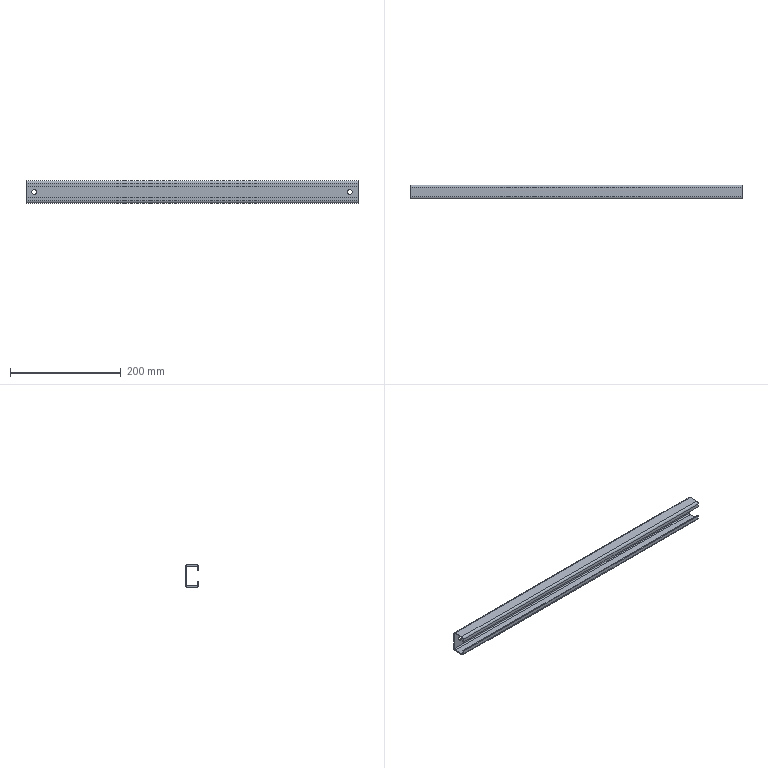Part | SolidWorks | features BaseBody 1 | 1 solid | 26 faces | box 600 x 25 x 40 mm | volume 115965 mm3 | plane 14 | cylinder 12 | commonest cylinder face diameters 4 x4 8 x4 9 x4
STEP:
#1=CARTESIAN_POINT('',(-285.,2.,4.5));
#2=VERTEX_POINT('',#1);
#3=CARTESIAN_POINT('',(-285.,2.,-4.5));
#4=VERTEX_POINT('',#3);
#5=CARTESIAN_POINT('',(-285.,2.,0.));
#6=DIRECTION('',(0.,-1.,0.));
#7=DIRECTION('',(0.,0.,-1.));
#8=AXIS2_PLACEMENT_3D('',#5,#6,#7);
#9=CIRCLE('',#8,4.5);
#10=EDGE_CURVE('',#2,#4,#9,.T.);
#11=ORIENTED_EDGE('',*,*,#10,.F.);
#12=CARTESIAN_POINT('',(-285.,0.,4.5));
#13=VERTEX_POINT('',#12);
#14=CARTESIAN_POINT('',(-285.,2.,4.5));
#15=DIRECTION('',(0.,-1.,0.));
#16=VECTOR('',#15,1000.);
#17=LINE('',#14,#16);
#18=EDGE_CURVE('',#2,#13,#17,.T.);
#19=ORIENTED_EDGE('',*,*,#18,.T.);
#20=CARTESIAN_POINT('',(-285.,0.,-4.5));
#21=VERTEX_POINT('',#20);
#22=CARTESIAN_POINT('',(-285.,0.,0.));
#23=DIRECTION('',(0.,-1.,0.));
#24=DIRECTION('',(0.,0.,-1.));
#25=AXIS2_PLACEMENT_3D('',#22,#23,#24);
#26=CIRCLE('',#25,4.5);
#27=EDGE_CURVE('',#13,#21,#26,.T.);
#28=ORIENTED_EDGE('',*,*,#27,.T.);
#29=CARTESIAN_POINT('',(-285.,2.,-4.5));
#30=DIRECTION('',(0.,-1.,0.));
#31=VECTOR('',#30,1000.);
#32=LINE('',#29,#31);
#33=EDGE_CURVE('',#4,#21,#32,.T.);
#34=ORIENTED_EDGE('',*,*,#33,.F.);
#35=EDGE_LOOP('',(#11,#19,#28,#34));
#36=FACE_OUTER_BOUND('',#35,.T.);
#37=CARTESIAN_POINT('',(-285.,2.,0.));
#38=DIRECTION('',(0.,-1.,0.));
#39=DIRECTION('',(0.,0.,-1.));
#40=AXIS2_PLACEMENT_3D('',#37,#38,#39);
#41=CYLINDRICAL_SURFACE('',#40,4.5);
#42=ADVANCED_FACE('',(#36),#41,.F.);
#43=CARTESIAN_POINT('',(285.,2.,4.5));
#44=VERTEX_POINT('',#43);
#45=CARTESIAN_POINT('',(285.,2.,-4.5));
#46=VERTEX_POINT('',#45);
#47=CARTESIAN_POINT('',(285.,2.,0.));
#48=DIRECTION('',(0.,-1.,0.));
#49=DIRECTION('',(0.,0.,-1.));
#50=AXIS2_PLACEMENT_3D('',#47,#48,#49);
#51=CIRCLE('',#50,4.5);
#52=EDGE_CURVE('',#44,#46,#51,.T.);
#53=ORIENTED_EDGE('',*,*,#52,.F.);
#54=CARTESIAN_POINT('',(285.,0.,4.5));
#55=VERTEX_POINT('',#54);
#56=CARTESIAN_POINT('',(285.,2.,4.5));
#57=DIRECTION('',(0.,-1.,0.));
#58=VECTOR('',#57,1000.);
#59=LINE('',#56,#58);
#60=EDGE_CURVE('',#44,#55,#59,.T.);
#61=ORIENTED_EDGE('',*,*,#60,.T.);
#62=CARTESIAN_POINT('',(285.,0.,-4.5));
#63=VERTEX_POINT('',#62);
#64=CARTESIAN_POINT('',(285.,0.,0.));
#65=DIRECTION('',(0.,-1.,0.));
#66=DIRECTION('',(0.,0.,-1.));
#67=AXIS2_PLACEMENT_3D('',#64,#65,#66);
#68=CIRCLE('',#67,4.5);
#69=EDGE_CURVE('',#55,#63,#68,.T.);
#70=ORIENTED_EDGE('',*,*,#69,.T.);
#71=CARTESIAN_POINT('',(285.,2.,-4.5));
#72=DIRECTION('',(0.,-1.,0.));
#73=VECTOR('',#72,1000.);
#74=LINE('',#71,#73);
#75=EDGE_CURVE('',#46,#63,#74,.T.);
#76=ORIENTED_EDGE('',*,*,#75,.F.);
#77=EDGE_LOOP('',(#53,#61,#70,#76));
#78=FACE_OUTER_BOUND('',#77,.T.);
#79=CARTESIAN_POINT('',(285.,2.,0.));
#80=DIRECTION('',(0.,-1.,0.));
#81=DIRECTION('',(0.,0.,-1.));
#82=AXIS2_PLACEMENT_3D('',#79,#80,#81);
#83=CYLINDRICAL_SURFACE('',#82,4.5);
#84=ADVANCED_FACE('',(#78),#83,.F.);
#85=CARTESIAN_POINT('',(-285.,0.,0.));
#86=DIRECTION('',(0.,-1.,0.));
#87=DIRECTION('',(0.,0.,-1.));
#88=AXIS2_PLACEMENT_3D('',#85,#86,#87);
#89=CIRCLE('',#88,4.5);
#90=EDGE_CURVE('',#21,#13,#89,.T.);
#91=ORIENTED_EDGE('',*,*,#90,.F.);
#92=ORIENTED_EDGE('',*,*,#27,.F.);
#93=EDGE_LOOP('',(#91,#92));
#94=FACE_BOUND('',#93,.T.);
#95=CARTESIAN_POINT('',(285.,0.,0.));
#96=DIRECTION('',(0.,-1.,0.));
#97=DIRECTION('',(0.,0.,-1.));
#98=AXIS2_PLACEMENT_3D('',#95,#96,#97);
#99=CIRCLE('',#98,4.5);
#100=EDGE_CURVE('',#63,#55,#99,.T.);
#101=ORIENTED_EDGE('',*,*,#100,.F.);
#102=ORIENTED_EDGE('',*,*,#69,.F.);
#103=EDGE_LOOP('',(#101,#102));
#104=FACE_BOUND('',#103,.T.);
#105=CARTESIAN_POINT('',(300.,0.,16.));
#106=VERTEX_POINT('',#105);
#107=CARTESIAN_POINT('',(300.,0.,-16.));
#108=VERTEX_POINT('',#107);
#109=CARTESIAN_POINT('',(300.,0.,0.));
#110=DIRECTION('',(0.,0.,-1.));
#111=VECTOR('',#110,1000.);
#112=LINE('',#109,#111);
#113=EDGE_CURVE('',#106,#108,#112,.T.);
#114=ORIENTED_EDGE('',*,*,#113,.F.);
#115=CARTESIAN_POINT('',(-300.,0.,16.));
#116=VERTEX_POINT('',#115);
#117=CARTESIAN_POINT('',(0.,0.,16.));
#118=DIRECTION('',(1.,0.,0.));
#119=VECTOR('',#118,1000.);
#120=LINE('',#117,#119);
#121=EDGE_CURVE('',#116,#106,#120,.T.);
#122=ORIENTED_EDGE('',*,*,#121,.F.);
#123=CARTESIAN_POINT('',(-300.,0.,-16.));
#124=VERTEX_POINT('',#123);
#125=CARTESIAN_POINT('',(-300.,0.,0.));
#126=DIRECTION('',(0.,0.,1.));
#127=VECTOR('',#126,1000.);
#128=LINE('',#125,#127);
#129=EDGE_CURVE('',#124,#116,#128,.T.);
#130=ORIENTED_EDGE('',*,*,#129,.F.);
#131=CARTESIAN_POINT('',(0.,0.,-16.));
#132=DIRECTION('',(-1.,0.,0.));
#133=VECTOR('',#132,1000.);
#134=LINE('',#131,#133);
#135=EDGE_CURVE('',#108,#124,#134,.T.);
#136=ORIENTED_EDGE('',*,*,#135,.F.);
#137=EDGE_LOOP('',(#114,#122,#130,#136));
#138=FACE_OUTER_BOUND('',#137,.T.);
#139=CARTESIAN_POINT('',(0.,0.,0.));
#140=DIRECTION('',(0.,1.,0.));
#141=DIRECTION('',(0.,0.,1.));
#142=AXIS2_PLACEMENT_3D('',#139,#140,#141);
#143=PLANE('',#142);
#144=ADVANCED_FACE('',(#94,#104,#138),#143,.F.);
#145=ORIENTED_EDGE('',*,*,#18,.F.);
#146=CARTESIAN_POINT('',(-285.,2.,0.));
#147=DIRECTION('',(0.,-1.,0.));
#148=DIRECTION('',(0.,0.,-1.));
#149=AXIS2_PLACEMENT_3D('',#146,#147,#148);
#150=CIRCLE('',#149,4.5);
#151=EDGE_CURVE('',#4,#2,#150,.T.);
#152=ORIENTED_EDGE('',*,*,#151,.F.);
#153=ORIENTED_EDGE('',*,*,#33,.T.);
#154=ORIENTED_EDGE('',*,*,#90,.T.);
#155=EDGE_LOOP('',(#145,#152,#153,#154));
#156=FACE_OUTER_BOUND('',#155,.T.);
#157=CARTESIAN_POINT('',(-285.,2.,0.));
#158=DIRECTION('',(0.,-1.,0.));
#159=DIRECTION('',(0.,0.,-1.));
#160=AXIS2_PLACEMENT_3D('',#157,#158,#159);
#161=CYLINDRICAL_SURFACE('',#160,4.5);
#162=ADVANCED_FACE('',(#156),#161,.F.);
#163=ORIENTED_EDGE('',*,*,#60,.F.);
#164=CARTESIAN_POINT('',(285.,2.,0.));
#165=DIRECTION('',(0.,-1.,0.));
#166=DIRECTION('',(0.,0.,-1.));
#167=AXIS2_PLACEMENT_3D('',#164,#165,#166);
#168=CIRCLE('',#167,4.5);
#169=EDGE_CURVE('',#46,#44,#168,.T.);
#170=ORIENTED_EDGE('',*,*,#169,.F.);
#171=ORIENTED_EDGE('',*,*,#75,.T.);
#172=ORIENTED_EDGE('',*,*,#100,.T.);
#173=EDGE_LOOP('',(#163,#170,#171,#172));
#174=FACE_OUTER_BOUND('',#173,.T.);
#175=CARTESIAN_POINT('',(285.,2.,0.));
#176=DIRECTION('',(0.,-1.,0.));
#177=DIRECTION('',(0.,0.,-1.));
#178=AXIS2_PLACEMENT_3D('',#175,#176,#177);
#179=CYLINDRICAL_SURFACE('',#178,4.5);
#180=ADVANCED_FACE('',(#174),#179,.F.);
#181=ORIENTED_EDGE('',*,*,#135,.T.);
#182=CARTESIAN_POINT('',(-300.,-2.,-18.));
#183=VERTEX_POINT('',#182);
#184=CARTESIAN_POINT('',(-300.,-2.,-16.));
#185=DIRECTION('',(1.,0.,0.));
#186=DIRECTION('',(0.,0.,-1.));
#187=AXIS2_PLACEMENT_3D('',#184,#185,#186);
#188=CIRCLE('',#187,2.);
#189=EDGE_CURVE('',#183,#124,#188,.T.);
#190=ORIENTED_EDGE('',*,*,#189,.F.);
#191=CARTESIAN_POINT('',(300.,-2.,-18.));
#192=VERTEX_POINT('',#191);
#193=CARTESIAN_POINT('',(-300.,-2.,-18.));
#194=DIRECTION('',(-1.,0.,0.));
#195=VECTOR('',#194,1000.);
#196=LINE('',#193,#195);
#197=EDGE_CURVE('',#192,#183,#196,.T.);
#198=ORIENTED_EDGE('',*,*,#197,.F.);
#199=CARTESIAN_POINT('',(300.,-2.,-16.));
#200=DIRECTION('',(-1.,0.,0.));
#201=DIRECTION('',(0.,0.,-1.));
#202=AXIS2_PLACEMENT_3D('',#199,#200,#201);
#203=CIRCLE('',#202,2.);
#204=EDGE_CURVE('',#108,#192,#203,.T.);
#205=ORIENTED_EDGE('',*,*,#204,.F.);
#206=EDGE_LOOP('',(#181,#190,#198,#205));
#207=FACE_OUTER_BOUND('',#206,.T.);
#208=CARTESIAN_POINT('',(-300.,-2.,-16.));
#209=DIRECTION('',(1.,0.,0.));
#210=DIRECTION('',(0.,0.,-1.));
#211=AXIS2_PLACEMENT_3D('',#208,#209,#210);
#212=CYLINDRICAL_SURFACE('',#211,2.);
#213=ADVANCED_FACE('',(#207),#212,.F.);
#214=CARTESIAN_POINT('',(300.,2.,16.));
#215=VERTEX_POINT('',#214);
#216=CARTESIAN_POINT('',(300.,2.,-16.));
#217=VERTEX_POINT('',#216);
#218=CARTESIAN_POINT('',(300.,2.,0.));
#219=DIRECTION('',(0.,0.,-1.));
#220=VECTOR('',#219,1000.);
#221=LINE('',#218,#220);
#222=EDGE_CURVE('',#215,#217,#221,.T.);
#223=ORIENTED_EDGE('',*,*,#222,.F.);
#224=CARTESIAN_POINT('',(300.,-2.,20.));
#225=VERTEX_POINT('',#224);
#226=CARTESIAN_POINT('',(300.,-2.,16.));
#227=DIRECTION('',(1.,0.,0.));
#228=DIRECTION('',(0.,0.,1.));
#229=AXIS2_PLACEMENT_3D('',#226,#227,#228);
#230=CIRCLE('',#229,4.);
#231=EDGE_CURVE('',#215,#225,#230,.T.);
#232=ORIENTED_EDGE('',*,*,#231,.T.);
#233=CARTESIAN_POINT('',(300.,-19.,20.));
#234=VERTEX_POINT('',#233);
#235=CARTESIAN_POINT('',(300.,-12.5,20.));
#236=DIRECTION('',(0.,-1.,0.));
#237=VECTOR('',#236,1000.);
#238=LINE('',#235,#237);
#239=EDGE_CURVE('',#225,#234,#238,.T.);
#240=ORIENTED_EDGE('',*,*,#239,.T.);
#241=CARTESIAN_POINT('',(300.,-23.,16.));
#242=VERTEX_POINT('',#241);
#243=CARTESIAN_POINT('',(300.,-19.,16.));
#244=DIRECTION('',(1.,0.,0.));
#245=DIRECTION('',(0.,0.,1.));
#246=AXIS2_PLACEMENT_3D('',#243,#244,#245);
#247=CIRCLE('',#246,4.);
#248=EDGE_CURVE('',#234,#242,#247,.T.);
#249=ORIENTED_EDGE('',*,*,#248,.T.);
#250=CARTESIAN_POINT('',(300.,-23.,10.));
#251=VERTEX_POINT('',#250);
#252=CARTESIAN_POINT('',(300.,-23.,13.));
#253=DIRECTION('',(0.,0.,-1.));
#254=VECTOR('',#253,1000.);
#255=LINE('',#252,#254);
#256=EDGE_CURVE('',#242,#251,#255,.T.);
#257=ORIENTED_EDGE('',*,*,#256,.T.);
#258=CARTESIAN_POINT('',(300.,-21.,10.));
#259=VERTEX_POINT('',#258);
#260=CARTESIAN_POINT('',(300.,-22.,10.));
#261=DIRECTION('',(0.,1.,0.));
#262=VECTOR('',#261,1000.);
#263=LINE('',#260,#262);
#264=EDGE_CURVE('',#251,#259,#263,.T.);
#265=ORIENTED_EDGE('',*,*,#264,.T.);
#266=CARTESIAN_POINT('',(300.,-21.,16.));
#267=VERTEX_POINT('',#266);
#268=CARTESIAN_POINT('',(300.,-21.,20.));
#269=DIRECTION('',(0.,0.,1.));
#270=VECTOR('',#269,1000.);
#271=LINE('',#268,#270);
#272=EDGE_CURVE('',#259,#267,#271,.T.);
#273=ORIENTED_EDGE('',*,*,#272,.T.);
#274=CARTESIAN_POINT('',(300.,-19.,18.));
#275=VERTEX_POINT('',#274);
#276=CARTESIAN_POINT('',(300.,-19.,16.));
#277=DIRECTION('',(-1.,0.,0.));
#278=DIRECTION('',(0.,0.,1.));
#279=AXIS2_PLACEMENT_3D('',#276,#277,#278);
#280=CIRCLE('',#279,2.);
#281=EDGE_CURVE('',#267,#275,#280,.T.);
#282=ORIENTED_EDGE('',*,*,#281,.T.);
#283=CARTESIAN_POINT('',(300.,-2.,18.));
#284=VERTEX_POINT('',#283);
#285=CARTESIAN_POINT('',(300.,2.,18.));
#286=DIRECTION('',(0.,1.,0.));
#287=VECTOR('',#286,1000.);
#288=LINE('',#285,#287);
#289=EDGE_CURVE('',#275,#284,#288,.T.);
#290=ORIENTED_EDGE('',*,*,#289,.T.);
#291=CARTESIAN_POINT('',(300.,-2.,16.));
#292=DIRECTION('',(-1.,0.,0.));
#293=DIRECTION('',(0.,0.,1.));
#294=AXIS2_PLACEMENT_3D('',#291,#292,#293);
#295=CIRCLE('',#294,2.);
#296=EDGE_CURVE('',#284,#106,#295,.T.);
#297=ORIENTED_EDGE('',*,*,#296,.T.);
#298=ORIENTED_EDGE('',*,*,#113,.T.);
#299=ORIENTED_EDGE('',*,*,#204,.T.);
#300=CARTESIAN_POINT('',(300.,-19.,-18.));
#301=VERTEX_POINT('',#300);
#302=CARTESIAN_POINT('',(300.,2.,-18.));
#303=DIRECTION('',(0.,-1.,0.));
#304=VECTOR('',#303,1000.);
#305=LINE('',#302,#304);
#306=EDGE_CURVE('',#192,#301,#305,.T.);
#307=ORIENTED_EDGE('',*,*,#306,.T.);
#308=CARTESIAN_POINT('',(300.,-21.,-16.));
#309=VERTEX_POINT('',#308);
#310=CARTESIAN_POINT('',(300.,-19.,-16.));
#311=DIRECTION('',(-1.,0.,0.));
#312=DIRECTION('',(0.,0.,-1.));
#313=AXIS2_PLACEMENT_3D('',#310,#311,#312);
#314=CIRCLE('',#313,2.);
#315=EDGE_CURVE('',#301,#309,#314,.T.);
#316=ORIENTED_EDGE('',*,*,#315,.T.);
#317=CARTESIAN_POINT('',(300.,-21.,-10.));
#318=VERTEX_POINT('',#317);
#319=CARTESIAN_POINT('',(300.,-21.,-20.));
#320=DIRECTION('',(0.,0.,1.));
#321=VECTOR('',#320,1000.);
#322=LINE('',#319,#321);
#323=EDGE_CURVE('',#309,#318,#322,.T.);
#324=ORIENTED_EDGE('',*,*,#323,.T.);
#325=CARTESIAN_POINT('',(300.,-23.,-10.));
#326=VERTEX_POINT('',#325);
#327=CARTESIAN_POINT('',(300.,-22.,-10.));
#328=DIRECTION('',(0.,-1.,0.));
#329=VECTOR('',#328,1000.);
#330=LINE('',#327,#329);
#331=EDGE_CURVE('',#318,#326,#330,.T.);
#332=ORIENTED_EDGE('',*,*,#331,.T.);
#333=CARTESIAN_POINT('',(300.,-23.,-16.));
#334=VERTEX_POINT('',#333);
#335=CARTESIAN_POINT('',(300.,-23.,-13.));
#336=DIRECTION('',(0.,0.,-1.));
#337=VECTOR('',#336,1000.);
#338=LINE('',#335,#337);
#339=EDGE_CURVE('',#326,#334,#338,.T.);
#340=ORIENTED_EDGE('',*,*,#339,.T.);
#341=CARTESIAN_POINT('',(300.,-19.,-20.));
#342=VERTEX_POINT('',#341);
#343=CARTESIAN_POINT('',(300.,-19.,-16.));
#344=DIRECTION('',(-1.,0.,0.));
#345=DIRECTION('',(0.,0.,-1.));
#346=AXIS2_PLACEMENT_3D('',#343,#344,#345);
#347=CIRCLE('',#346,4.);
#348=EDGE_CURVE('',#342,#334,#347,.T.);
#349=ORIENTED_EDGE('',*,*,#348,.F.);
#350=CARTESIAN_POINT('',(300.,-2.,-20.));
#351=VERTEX_POINT('',#350);
#352=CARTESIAN_POINT('',(300.,-12.5,-20.));
#353=DIRECTION('',(0.,1.,0.));
#354=VECTOR('',#353,1000.);
#355=LINE('',#352,#354);
#356=EDGE_CURVE('',#342,#351,#355,.T.);
#357=ORIENTED_EDGE('',*,*,#356,.T.);
#358=CARTESIAN_POINT('',(300.,-2.,-16.));
#359=DIRECTION('',(-1.,0.,0.));
#360=DIRECTION('',(0.,0.,-1.));
#361=AXIS2_PLACEMENT_3D('',#358,#359,#360);
#362=CIRCLE('',#361,4.);
#363=EDGE_CURVE('',#217,#351,#362,.T.);
#364=ORIENTED_EDGE('',*,*,#363,.F.);
#365=EDGE_LOOP('',(#223,#232,#240,#249,#257,#265,#273,#282,#290,#297,#298,#299,#307,#316,#324,#332,#340,#349,#357,#364));
#366=FACE_OUTER_BOUND('',#365,.T.);
#367=CARTESIAN_POINT('',(300.,1.,0.));
#368=DIRECTION('',(-1.,0.,0.));
#369=DIRECTION('',(0.,0.,1.));
#370=AXIS2_PLACEMENT_3D('',#367,#368,#369);
#371=PLANE('',#370);
#372=ADVANCED_FACE('',(#366),#371,.F.);
#373=ORIENTED_EDGE('',*,*,#121,.T.);
#374=ORIENTED_EDGE('',*,*,#296,.F.);
#375=CARTESIAN_POINT('',(-300.,-2.,18.));
#376=VERTEX_POINT('',#375);
#377=CARTESIAN_POINT('',(300.,-2.,18.));
#378=DIRECTION('',(1.,0.,0.));
#379=VECTOR('',#378,1000.);
#380=LINE('',#377,#379);
#381=EDGE_CURVE('',#376,#284,#380,.T.);
#382=ORIENTED_EDGE('',*,*,#381,.F.);
#383=CARTESIAN_POINT('',(-300.,-2.,16.));
#384=DIRECTION('',(1.,0.,0.));
#385=DIRECTION('',(0.,0.,1.));
#386=AXIS2_PLACEMENT_3D('',#383,#384,#385);
#387=CIRCLE('',#386,2.);
#388=EDGE_CURVE('',#116,#376,#387,.T.);
#389=ORIENTED_EDGE('',*,*,#388,.F.);
#390=EDGE_LOOP('',(#373,#374,#382,#389));
#391=FACE_OUTER_BOUND('',#390,.T.);
#392=CARTESIAN_POINT('',(300.,-2.,16.));
#393=DIRECTION('',(-1.,0.,0.));
#394=DIRECTION('',(0.,0.,1.));
#395=AXIS2_PLACEMENT_3D('',#392,#393,#394);
#396=CYLINDRICAL_SURFACE('',#395,2.);
#397=ADVANCED_FACE('',(#391),#396,.F.);
#398=CARTESIAN_POINT('',(-300.,2.,-16.));
#399=VERTEX_POINT('',#398);
#400=CARTESIAN_POINT('',(-300.,2.,16.));
#401=VERTEX_POINT('',#400);
#402=CARTESIAN_POINT('',(-300.,2.,0.));
#403=DIRECTION('',(0.,0.,1.));
#404=VECTOR('',#403,1000.);
#405=LINE('',#402,#404);
#406=EDGE_CURVE('',#399,#401,#405,.T.);
#407=ORIENTED_EDGE('',*,*,#406,.F.);
#408=CARTESIAN_POINT('',(-300.,-2.,-20.));
#409=VERTEX_POINT('',#408);
#410=CARTESIAN_POINT('',(-300.,-2.,-16.));
#411=DIRECTION('',(-1.,0.,0.));
#412=DIRECTION('',(0.,0.,-1.));
#413=AXIS2_PLACEMENT_3D('',#410,#411,#412);
#414=CIRCLE('',#413,4.);
#415=EDGE_CURVE('',#399,#409,#414,.T.);
#416=ORIENTED_EDGE('',*,*,#415,.T.);
#417=CARTESIAN_POINT('',(-300.,-19.,-20.));
#418=VERTEX_POINT('',#417);
#419=CARTESIAN_POINT('',(-300.,-12.5,-20.));
#420=DIRECTION('',(0.,-1.,0.));
#421=VECTOR('',#420,1000.);
#422=LINE('',#419,#421);
#423=EDGE_CURVE('',#409,#418,#422,.T.);
#424=ORIENTED_EDGE('',*,*,#423,.T.);
#425=CARTESIAN_POINT('',(-300.,-23.,-16.));
#426=VERTEX_POINT('',#425);
#427=CARTESIAN_POINT('',(-300.,-19.,-16.));
#428=DIRECTION('',(-1.,0.,0.));
#429=DIRECTION('',(0.,0.,-1.));
#430=AXIS2_PLACEMENT_3D('',#427,#428,#429);
#431=CIRCLE('',#430,4.);
#432=EDGE_CURVE('',#418,#426,#431,.T.);
#433=ORIENTED_EDGE('',*,*,#432,.T.);
#434=CARTESIAN_POINT('',(-300.,-23.,-10.));
#435=VERTEX_POINT('',#434);
#436=CARTESIAN_POINT('',(-300.,-23.,-13.));
#437=DIRECTION('',(0.,0.,1.));
#438=VECTOR('',#437,1000.);
#439=LINE('',#436,#438);
#440=EDGE_CURVE('',#426,#435,#439,.T.);
#441=ORIENTED_EDGE('',*,*,#440,.T.);
#442=CARTESIAN_POINT('',(-300.,-21.,-10.));
#443=VERTEX_POINT('',#442);
#444=CARTESIAN_POINT('',(-300.,-22.,-10.));
#445=DIRECTION('',(0.,1.,0.));
#446=VECTOR('',#445,1000.);
#447=LINE('',#444,#446);
#448=EDGE_CURVE('',#435,#443,#447,.T.);
#449=ORIENTED_EDGE('',*,*,#448,.T.);
#450=CARTESIAN_POINT('',(-300.,-21.,-16.));
#451=VERTEX_POINT('',#450);
#452=CARTESIAN_POINT('',(-300.,-21.,-20.));
#453=DIRECTION('',(0.,0.,-1.));
#454=VECTOR('',#453,1000.);
#455=LINE('',#452,#454);
#456=EDGE_CURVE('',#443,#451,#455,.T.);
#457=ORIENTED_EDGE('',*,*,#456,.T.);
#458=CARTESIAN_POINT('',(-300.,-19.,-18.));
#459=VERTEX_POINT('',#458);
#460=CARTESIAN_POINT('',(-300.,-19.,-16.));
#461=DIRECTION('',(1.,0.,0.));
#462=DIRECTION('',(0.,0.,-1.));
#463=AXIS2_PLACEMENT_3D('',#460,#461,#462);
#464=CIRCLE('',#463,2.);
#465=EDGE_CURVE('',#451,#459,#464,.T.);
#466=ORIENTED_EDGE('',*,*,#465,.T.);
#467=CARTESIAN_POINT('',(-300.,2.,-18.));
#468=DIRECTION('',(0.,1.,0.));
#469=VECTOR('',#468,1000.);
#470=LINE('',#467,#469);
#471=EDGE_CURVE('',#459,#183,#470,.T.);
#472=ORIENTED_EDGE('',*,*,#471,.T.);
#473=ORIENTED_EDGE('',*,*,#189,.T.);
#474=ORIENTED_EDGE('',*,*,#129,.T.);
#475=ORIENTED_EDGE('',*,*,#388,.T.);
#476=CARTESIAN_POINT('',(-300.,-19.,18.));
#477=VERTEX_POINT('',#476);
#478=CARTESIAN_POINT('',(-300.,2.,18.));
#479=DIRECTION('',(0.,-1.,0.));
#480=VECTOR('',#479,1000.);
#481=LINE('',#478,#480);
#482=EDGE_CURVE('',#376,#477,#481,.T.);
#483=ORIENTED_EDGE('',*,*,#482,.T.);
#484=CARTESIAN_POINT('',(-300.,-21.,16.));
#485=VERTEX_POINT('',#484);
#486=CARTESIAN_POINT('',(-300.,-19.,16.));
#487=DIRECTION('',(1.,0.,0.));
#488=DIRECTION('',(0.,0.,1.));
#489=AXIS2_PLACEMENT_3D('',#486,#487,#488);
#490=CIRCLE('',#489,2.);
#491=EDGE_CURVE('',#477,#485,#490,.T.);
#492=ORIENTED_EDGE('',*,*,#491,.T.);
#493=CARTESIAN_POINT('',(-300.,-21.,10.));
#494=VERTEX_POINT('',#493);
#495=CARTESIAN_POINT('',(-300.,-21.,20.));
#496=DIRECTION('',(0.,0.,-1.));
#497=VECTOR('',#496,1000.);
#498=LINE('',#495,#497);
#499=EDGE_CURVE('',#485,#494,#498,.T.);
#500=ORIENTED_EDGE('',*,*,#499,.T.);
#501=CARTESIAN_POINT('',(-300.,-23.,10.));
#502=VERTEX_POINT('',#501);
#503=CARTESIAN_POINT('',(-300.,-22.,10.));
#504=DIRECTION('',(0.,-1.,0.));
#505=VECTOR('',#504,1000.);
#506=LINE('',#503,#505);
#507=EDGE_CURVE('',#494,#502,#506,.T.);
#508=ORIENTED_EDGE('',*,*,#507,.T.);
#509=CARTESIAN_POINT('',(-300.,-23.,16.));
#510=VERTEX_POINT('',#509);
#511=CARTESIAN_POINT('',(-300.,-23.,13.));
#512=DIRECTION('',(0.,0.,1.));
#513=VECTOR('',#512,1000.);
#514=LINE('',#511,#513);
#515=EDGE_CURVE('',#502,#510,#514,.T.);
#516=ORIENTED_EDGE('',*,*,#515,.T.);
#517=CARTESIAN_POINT('',(-300.,-19.,20.));
#518=VERTEX_POINT('',#517);
#519=CARTESIAN_POINT('',(-300.,-19.,16.));
#520=DIRECTION('',(1.,0.,0.));
#521=DIRECTION('',(0.,0.,1.));
#522=AXIS2_PLACEMENT_3D('',#519,#520,#521);
#523=CIRCLE('',#522,4.);
#524=EDGE_CURVE('',#518,#510,#523,.T.);
#525=ORIENTED_EDGE('',*,*,#524,.F.);
#526=CARTESIAN_POINT('',(-300.,-2.,20.));
#527=VERTEX_POINT('',#526);
#528=CARTESIAN_POINT('',(-300.,-12.5,20.));
#529=DIRECTION('',(0.,1.,0.));
#530=VECTOR('',#529,1000.);
#531=LINE('',#528,#530);
#532=EDGE_CURVE('',#518,#527,#531,.T.);
#533=ORIENTED_EDGE('',*,*,#532,.T.);
#534=CARTESIAN_POINT('',(-300.,-2.,16.));
#535=DIRECTION('',(1.,0.,0.));
#536=DIRECTION('',(0.,0.,1.));
#537=AXIS2_PLACEMENT_3D('',#534,#535,#536);
#538=CIRCLE('',#537,4.);
#539=EDGE_CURVE('',#401,#527,#538,.T.);
#540=ORIENTED_EDGE('',*,*,#539,.F.);
#541=EDGE_LOOP('',(#407,#416,#424,#433,#441,#449,#457,#466,#472,#473,#474,#475,#483,#492,#500,#508,#516,#525,#533,#540));
#542=FACE_OUTER_BOUND('',#541,.T.);
#543=CARTESIAN_POINT('',(-300.,1.,0.));
#544=DIRECTION('',(1.,0.,0.));
#545=DIRECTION('',(0.,0.,-1.));
#546=AXIS2_PLACEMENT_3D('',#543,#544,#545);
#547=PLANE('',#546);
#548=ADVANCED_FACE('',(#542),#547,.F.);
#549=ORIENTED_EDGE('',*,*,#151,.T.);
#550=ORIENTED_EDGE('',*,*,#10,.T.);
#551=EDGE_LOOP('',(#549,#550));
#552=FACE_BOUND('',#551,.T.);
#553=ORIENTED_EDGE('',*,*,#169,.T.);
#554=ORIENTED_EDGE('',*,*,#52,.T.);
#555=EDGE_LOOP('',(#553,#554));
#556=FACE_BOUND('',#555,.T.);
#557=CARTESIAN_POINT('',(0.,2.,-16.));
#558=DIRECTION('',(-1.,0.,0.));
#559=VECTOR('',#558,1000.);
#560=LINE('',#557,#559);
#561=EDGE_CURVE('',#217,#399,#560,.T.);
#562=ORIENTED_EDGE('',*,*,#561,.T.);
#563=ORIENTED_EDGE('',*,*,#406,.T.);
#564=CARTESIAN_POINT('',(0.,2.,16.));
#565=DIRECTION('',(1.,0.,0.));
#566=VECTOR('',#565,1000.);
#567=LINE('',#564,#566);
#568=EDGE_CURVE('',#401,#215,#567,.T.);
#569=ORIENTED_EDGE('',*,*,#568,.T.);
#570=ORIENTED_EDGE('',*,*,#222,.T.);
#571=EDGE_LOOP('',(#562,#563,#569,#570));
#572=FACE_OUTER_BOUND('',#571,.T.);
#573=CARTESIAN_POINT('',(0.,2.,0.));
#574=DIRECTION('',(0.,1.,0.));
#575=DIRECTION('',(0.,0.,1.));
#576=AXIS2_PLACEMENT_3D('',#573,#574,#575);
#577=PLANE('',#576);
#578=ADVANCED_FACE('',(#552,#556,#572),#577,.T.);
#579=ORIENTED_EDGE('',*,*,#471,.F.);
#580=CARTESIAN_POINT('',(300.,-19.,-18.));
#581=DIRECTION('',(-1.,0.,0.));
#582=VECTOR('',#581,1000.);
#583=LINE('',#580,#582);
#584=EDGE_CURVE('',#301,#459,#583,.T.);
#585=ORIENTED_EDGE('',*,*,#584,.F.);
#586=ORIENTED_EDGE('',*,*,#306,.F.);
#587=ORIENTED_EDGE('',*,*,#197,.T.);
#588=EDGE_LOOP('',(#579,#585,#586,#587));
#589=FACE_OUTER_BOUND('',#588,.T.);
#590=CARTESIAN_POINT('',(300.,2.,-18.));
#591=DIRECTION('',(0.,0.,-1.));
#592=DIRECTION('',(-1.,0.,0.));
#593=AXIS2_PLACEMENT_3D('',#590,#591,#592);
#594=PLANE('',#593);
#595=ADVANCED_FACE('',(#589),#594,.F.);
#596=ORIENTED_EDGE('',*,*,#289,.F.);
#597=CARTESIAN_POINT('',(-300.,-19.,18.));
#598=DIRECTION('',(1.,0.,0.));
#599=VECTOR('',#598,1000.);
#600=LINE('',#597,#599);
#601=EDGE_CURVE('',#477,#275,#600,.T.);
#602=ORIENTED_EDGE('',*,*,#601,.F.);
#603=ORIENTED_EDGE('',*,*,#482,.F.);
#604=ORIENTED_EDGE('',*,*,#381,.T.);
#605=EDGE_LOOP('',(#596,#602,#603,#604));
#606=FACE_OUTER_BOUND('',#605,.T.);
#607=CARTESIAN_POINT('',(-300.,2.,18.));
#608=DIRECTION('',(0.,0.,1.));
#609=DIRECTION('',(1.,0.,0.));
#610=AXIS2_PLACEMENT_3D('',#607,#608,#609);
#611=PLANE('',#610);
#612=ADVANCED_FACE('',(#606),#611,.F.);
#613=ORIENTED_EDGE('',*,*,#363,.T.);
#614=CARTESIAN_POINT('',(-300.,-2.,-20.));
#615=DIRECTION('',(-1.,0.,0.));
#616=VECTOR('',#615,1000.);
#617=LINE('',#614,#616);
#618=EDGE_CURVE('',#351,#409,#617,.T.);
#619=ORIENTED_EDGE('',*,*,#618,.T.);
#620=ORIENTED_EDGE('',*,*,#415,.F.);
#621=ORIENTED_EDGE('',*,*,#561,.F.);
#622=EDGE_LOOP('',(#613,#619,#620,#621));
#623=FACE_OUTER_BOUND('',#622,.T.);
#624=CARTESIAN_POINT('',(-300.,-2.,-16.));
#625=DIRECTION('',(1.,0.,0.));
#626=DIRECTION('',(0.,0.,-1.));
#627=AXIS2_PLACEMENT_3D('',#624,#625,#626);
#628=CYLINDRICAL_SURFACE('',#627,4.);
#629=ADVANCED_FACE('',(#623),#628,.T.);
#630=ORIENTED_EDGE('',*,*,#539,.T.);
#631=CARTESIAN_POINT('',(300.,-2.,20.));
#632=DIRECTION('',(1.,0.,0.));
#633=VECTOR('',#632,1000.);
#634=LINE('',#631,#633);
#635=EDGE_CURVE('',#527,#225,#634,.T.);
#636=ORIENTED_EDGE('',*,*,#635,.T.);
#637=ORIENTED_EDGE('',*,*,#231,.F.);
#638=ORIENTED_EDGE('',*,*,#568,.F.);
#639=EDGE_LOOP('',(#630,#636,#637,#638));
#640=FACE_OUTER_BOUND('',#639,.T.);
#641=CARTESIAN_POINT('',(300.,-2.,16.));
#642=DIRECTION('',(-1.,0.,0.));
#643=DIRECTION('',(0.,0.,1.));
#644=AXIS2_PLACEMENT_3D('',#641,#642,#643);
#645=CYLINDRICAL_SURFACE('',#644,4.);
#646=ADVANCED_FACE('',(#640),#645,.T.);
#647=ORIENTED_EDGE('',*,*,#584,.T.);
#648=ORIENTED_EDGE('',*,*,#465,.F.);
#649=CARTESIAN_POINT('',(-300.,-21.,-16.));
#650=DIRECTION('',(-1.,0.,0.));
#651=VECTOR('',#650,1000.);
#652=LINE('',#649,#651);
#653=EDGE_CURVE('',#309,#451,#652,.T.);
#654=ORIENTED_EDGE('',*,*,#653,.F.);
#655=ORIENTED_EDGE('',*,*,#315,.F.);
#656=EDGE_LOOP('',(#647,#648,#654,#655));
#657=FACE_OUTER_BOUND('',#656,.T.);
#658=CARTESIAN_POINT('',(-300.,-19.,-16.));
#659=DIRECTION('',(1.,0.,0.));
#660=DIRECTION('',(0.,0.,-1.));
#661=AXIS2_PLACEMENT_3D('',#658,#659,#660);
#662=CYLINDRICAL_SURFACE('',#661,2.);
#663=ADVANCED_FACE('',(#657),#662,.F.);
#664=ORIENTED_EDGE('',*,*,#601,.T.);
#665=ORIENTED_EDGE('',*,*,#281,.F.);
#666=CARTESIAN_POINT('',(300.,-21.,16.));
#667=DIRECTION('',(1.,0.,0.));
#668=VECTOR('',#667,1000.);
#669=LINE('',#666,#668);
#670=EDGE_CURVE('',#485,#267,#669,.T.);
#671=ORIENTED_EDGE('',*,*,#670,.F.);
#672=ORIENTED_EDGE('',*,*,#491,.F.);
#673=EDGE_LOOP('',(#664,#665,#671,#672));
#674=FACE_OUTER_BOUND('',#673,.T.);
#675=CARTESIAN_POINT('',(300.,-19.,16.));
#676=DIRECTION('',(-1.,0.,0.));
#677=DIRECTION('',(0.,0.,1.));
#678=AXIS2_PLACEMENT_3D('',#675,#676,#677);
#679=CYLINDRICAL_SURFACE('',#678,2.);
#680=ADVANCED_FACE('',(#674),#679,.F.);
#681=ORIENTED_EDGE('',*,*,#618,.F.);
#682=ORIENTED_EDGE('',*,*,#356,.F.);
#683=CARTESIAN_POINT('',(300.,-19.,-20.));
#684=DIRECTION('',(-1.,0.,0.));
#685=VECTOR('',#684,1000.);
#686=LINE('',#683,#685);
#687=EDGE_CURVE('',#342,#418,#686,.T.);
#688=ORIENTED_EDGE('',*,*,#687,.T.);
#689=ORIENTED_EDGE('',*,*,#423,.F.);
#690=EDGE_LOOP('',(#681,#682,#688,#689));
#691=FACE_OUTER_BOUND('',#690,.T.);
#692=CARTESIAN_POINT('',(300.,2.,-20.));
#693=DIRECTION('',(0.,0.,-1.));
#694=DIRECTION('',(-1.,0.,0.));
#695=AXIS2_PLACEMENT_3D('',#692,#693,#694);
#696=PLANE('',#695);
#697=ADVANCED_FACE('',(#691),#696,.T.);
#698=ORIENTED_EDGE('',*,*,#635,.F.);
#699=ORIENTED_EDGE('',*,*,#532,.F.);
#700=CARTESIAN_POINT('',(-300.,-19.,20.));
#701=DIRECTION('',(1.,0.,0.));
#702=VECTOR('',#701,1000.);
#703=LINE('',#700,#702);
#704=EDGE_CURVE('',#518,#234,#703,.T.);
#705=ORIENTED_EDGE('',*,*,#704,.T.);
#706=ORIENTED_EDGE('',*,*,#239,.F.);
#707=EDGE_LOOP('',(#698,#699,#705,#706));
#708=FACE_OUTER_BOUND('',#707,.T.);
#709=CARTESIAN_POINT('',(-300.,2.,20.));
#710=DIRECTION('',(0.,0.,1.));
#711=DIRECTION('',(1.,0.,0.));
#712=AXIS2_PLACEMENT_3D('',#709,#710,#711);
#713=PLANE('',#712);
#714=ADVANCED_FACE('',(#708),#713,.T.);
#715=ORIENTED_EDGE('',*,*,#456,.F.);
#716=CARTESIAN_POINT('',(300.,-21.,-10.));
#717=DIRECTION('',(-1.,0.,0.));
#718=VECTOR('',#717,1000.);
#719=LINE('',#716,#718);
#720=EDGE_CURVE('',#318,#443,#719,.T.);
#721=ORIENTED_EDGE('',*,*,#720,.F.);
#722=ORIENTED_EDGE('',*,*,#323,.F.);
#723=ORIENTED_EDGE('',*,*,#653,.T.);
#724=EDGE_LOOP('',(#715,#721,#722,#723));
#725=FACE_OUTER_BOUND('',#724,.T.);
#726=CARTESIAN_POINT('',(300.,-21.,-20.));
#727=DIRECTION('',(0.,-1.,0.));
#728=DIRECTION('',(0.,0.,-1.));
#729=AXIS2_PLACEMENT_3D('',#726,#727,#728);
#730=PLANE('',#729);
#731=ADVANCED_FACE('',(#725),#730,.F.);
#732=ORIENTED_EDGE('',*,*,#272,.F.);
#733=CARTESIAN_POINT('',(-300.,-21.,10.));
#734=DIRECTION('',(1.,0.,0.));
#735=VECTOR('',#734,1000.);
#736=LINE('',#733,#735);
#737=EDGE_CURVE('',#494,#259,#736,.T.);
#738=ORIENTED_EDGE('',*,*,#737,.F.);
#739=ORIENTED_EDGE('',*,*,#499,.F.);
#740=ORIENTED_EDGE('',*,*,#670,.T.);
#741=EDGE_LOOP('',(#732,#738,#739,#740));
#742=FACE_OUTER_BOUND('',#741,.T.);
#743=CARTESIAN_POINT('',(-300.,-21.,20.));
#744=DIRECTION('',(0.,-1.,0.));
#745=DIRECTION('',(0.,0.,-1.));
#746=AXIS2_PLACEMENT_3D('',#743,#744,#745);
#747=PLANE('',#746);
#748=ADVANCED_FACE('',(#742),#747,.F.);
#749=ORIENTED_EDGE('',*,*,#348,.T.);
#750=CARTESIAN_POINT('',(-300.,-23.,-16.));
#751=DIRECTION('',(-1.,0.,0.));
#752=VECTOR('',#751,1000.);
#753=LINE('',#750,#752);
#754=EDGE_CURVE('',#334,#426,#753,.T.);
#755=ORIENTED_EDGE('',*,*,#754,.T.);
#756=ORIENTED_EDGE('',*,*,#432,.F.);
#757=ORIENTED_EDGE('',*,*,#687,.F.);
#758=EDGE_LOOP('',(#749,#755,#756,#757));
#759=FACE_OUTER_BOUND('',#758,.T.);
#760=CARTESIAN_POINT('',(-300.,-19.,-16.));
#761=DIRECTION('',(1.,0.,0.));
#762=DIRECTION('',(0.,0.,-1.));
#763=AXIS2_PLACEMENT_3D('',#760,#761,#762);
#764=CYLINDRICAL_SURFACE('',#763,4.);
#765=ADVANCED_FACE('',(#759),#764,.T.);
#766=ORIENTED_EDGE('',*,*,#524,.T.);
#767=CARTESIAN_POINT('',(300.,-23.,16.));
#768=DIRECTION('',(1.,0.,0.));
#769=VECTOR('',#768,1000.);
#770=LINE('',#767,#769);
#771=EDGE_CURVE('',#510,#242,#770,.T.);
#772=ORIENTED_EDGE('',*,*,#771,.T.);
#773=ORIENTED_EDGE('',*,*,#248,.F.);
#774=ORIENTED_EDGE('',*,*,#704,.F.);
#775=EDGE_LOOP('',(#766,#772,#773,#774));
#776=FACE_OUTER_BOUND('',#775,.T.);
#777=CARTESIAN_POINT('',(300.,-19.,16.));
#778=DIRECTION('',(-1.,0.,0.));
#779=DIRECTION('',(0.,0.,1.));
#780=AXIS2_PLACEMENT_3D('',#777,#778,#779);
#781=CYLINDRICAL_SURFACE('',#780,4.);
#782=ADVANCED_FACE('',(#776),#781,.T.);
#783=ORIENTED_EDGE('',*,*,#448,.F.);
#784=CARTESIAN_POINT('',(0.,-23.,-10.));
#785=DIRECTION('',(1.,0.,0.));
#786=VECTOR('',#785,1000.);
#787=LINE('',#784,#786);
#788=EDGE_CURVE('',#435,#326,#787,.T.);
#789=ORIENTED_EDGE('',*,*,#788,.T.);
#790=ORIENTED_EDGE('',*,*,#331,.F.);
#791=ORIENTED_EDGE('',*,*,#720,.T.);
#792=EDGE_LOOP('',(#783,#789,#790,#791));
#793=FACE_OUTER_BOUND('',#792,.T.);
#794=CARTESIAN_POINT('',(0.,-22.,-10.));
#795=DIRECTION('',(0.,0.,1.));
#796=DIRECTION('',(1.,0.,0.));
#797=AXIS2_PLACEMENT_3D('',#794,#795,#796);
#798=PLANE('',#797);
#799=ADVANCED_FACE('',(#793),#798,.T.);
#800=ORIENTED_EDGE('',*,*,#264,.F.);
#801=CARTESIAN_POINT('',(0.,-23.,10.));
#802=DIRECTION('',(-1.,0.,0.));
#803=VECTOR('',#802,1000.);
#804=LINE('',#801,#803);
#805=EDGE_CURVE('',#251,#502,#804,.T.);
#806=ORIENTED_EDGE('',*,*,#805,.T.);
#807=ORIENTED_EDGE('',*,*,#507,.F.);
#808=ORIENTED_EDGE('',*,*,#737,.T.);
#809=EDGE_LOOP('',(#800,#806,#807,#808));
#810=FACE_OUTER_BOUND('',#809,.T.);
#811=CARTESIAN_POINT('',(0.,-22.,10.));
#812=DIRECTION('',(0.,0.,-1.));
#813=DIRECTION('',(-1.,0.,0.));
#814=AXIS2_PLACEMENT_3D('',#811,#812,#813);
#815=PLANE('',#814);
#816=ADVANCED_FACE('',(#810),#815,.T.);
#817=ORIENTED_EDGE('',*,*,#754,.F.);
#818=ORIENTED_EDGE('',*,*,#339,.F.);
#819=ORIENTED_EDGE('',*,*,#788,.F.);
#820=ORIENTED_EDGE('',*,*,#440,.F.);
#821=EDGE_LOOP('',(#817,#818,#819,#820));
#822=FACE_OUTER_BOUND('',#821,.T.);
#823=CARTESIAN_POINT('',(300.,-23.,-20.));
#824=DIRECTION('',(0.,-1.,0.));
#825=DIRECTION('',(0.,0.,-1.));
#826=AXIS2_PLACEMENT_3D('',#823,#824,#825);
#827=PLANE('',#826);
#828=ADVANCED_FACE('',(#822),#827,.T.);
#829=ORIENTED_EDGE('',*,*,#771,.F.);
#830=ORIENTED_EDGE('',*,*,#515,.F.);
#831=ORIENTED_EDGE('',*,*,#805,.F.);
#832=ORIENTED_EDGE('',*,*,#256,.F.);
#833=EDGE_LOOP('',(#829,#830,#831,#832));
#834=FACE_OUTER_BOUND('',#833,.T.);
#835=CARTESIAN_POINT('',(-300.,-23.,20.));
#836=DIRECTION('',(0.,-1.,0.));
#837=DIRECTION('',(0.,0.,-1.));
#838=AXIS2_PLACEMENT_3D('',#835,#836,#837);
#839=PLANE('',#838);
#840=ADVANCED_FACE('',(#834),#839,.T.);
#841=CLOSED_SHELL('',(#42,#84,#144,#162,#180,#213,#372,#397,#548,#578,#595,#612,#629,#646,#663,#680,#697,#714,#731,#748,#765,#782,#799,#816,#828,#840));
#842=MANIFOLD_SOLID_BREP('',#841);
#843=CARTESIAN_POINT('',(0.,0.,0.));
#844=DIRECTION('',(0.,0.,1.));
#845=DIRECTION('',(1.,0.,0.));
#846=AXIS2_PLACEMENT_3D('',#843,#844,#845);
#847=(LENGTH_UNIT()NAMED_UNIT(*)SI_UNIT(.MILLI.,.METRE.));
#848=UNCERTAINTY_MEASURE_WITH_UNIT(LENGTH_MEASURE(0.00001),#847,'','');
#849=(NAMED_UNIT(*)PLANE_ANGLE_UNIT()SI_UNIT($,.RADIAN.));
#850=(NAMED_UNIT(*)SI_UNIT($,.STERADIAN.)SOLID_ANGLE_UNIT());
#851=(GEOMETRIC_REPRESENTATION_CONTEXT(3)GLOBAL_UNCERTAINTY_ASSIGNED_CONTEXT((#848))GLOBAL_UNIT_ASSIGNED_CONTEXT((#847,#849,#850))REPRESENTATION_CONTEXT('',''));
#852=ADVANCED_BREP_SHAPE_REPRESENTATION('',(#842,#846),#851);